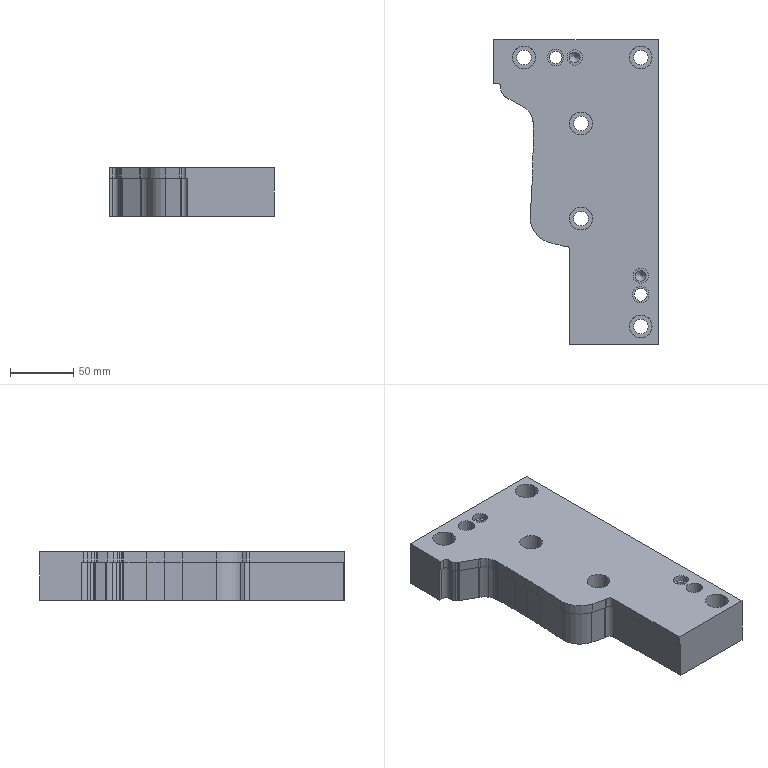Part | STEP file | lll_id270_x_t | 1 solid | 85 faces | box 130 x 240 x 38 mm | volume 814824 mm3 | cylinder 61 | plane 22 | cone 2 | commonest cylinder face diameters 11.509 x5 18.008 x5 6 x3 13 x3 8.506 x2 9 x2